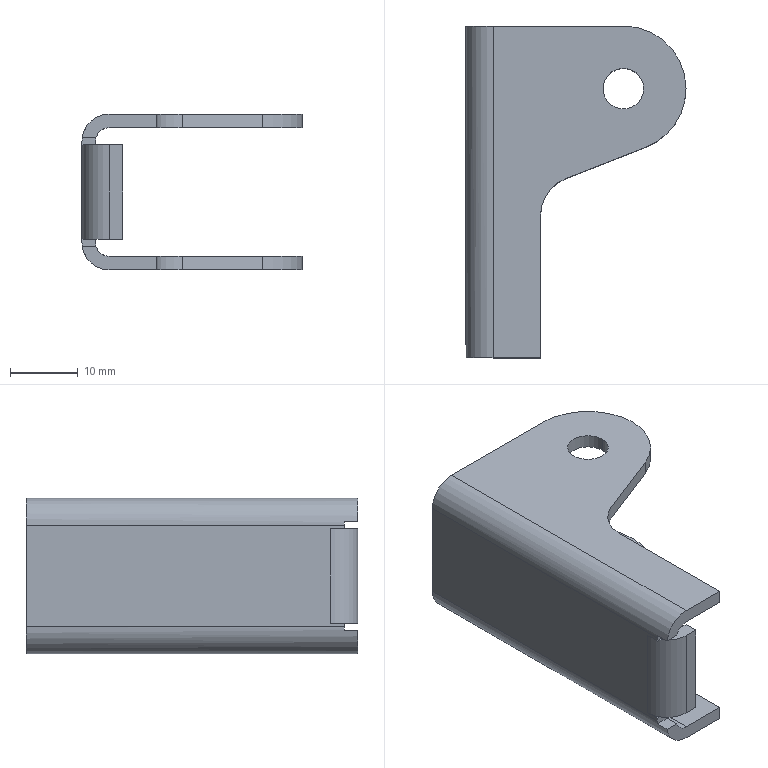Part | SolidWorks | features BaseBody 1 | 1 solid | 40 faces | box 32.5 x 49 x 23 mm | volume 5331 mm3 | plane 24 | cylinder 16 | commonest cylinder face diameters 6 x4 18.5 x4 4 x3 8 x3 12 x2
STEP:
#1=CARTESIAN_POINT('',(0.5359,2.,-7.));
#2=VERTEX_POINT('',#1);
#3=CARTESIAN_POINT('',(0.,4.,-7.));
#4=VERTEX_POINT('',#3);
#5=CARTESIAN_POINT('',(4.,4.,-7.));
#6=DIRECTION('',(0.,0.,-1.));
#7=DIRECTION('',(-0.866,-0.5,0.));
#8=AXIS2_PLACEMENT_3D('',#5,#6,#7);
#9=CIRCLE('',#8,4.);
#10=EDGE_CURVE('',#2,#4,#9,.T.);
#11=ORIENTED_EDGE('',*,*,#10,.T.);
#12=CARTESIAN_POINT('',(0.,2.,-7.));
#13=VERTEX_POINT('',#12);
#14=CARTESIAN_POINT('',(0.,4.,-7.));
#15=DIRECTION('',(0.,-1.,0.));
#16=VECTOR('',#15,1000.);
#17=LINE('',#14,#16);
#18=EDGE_CURVE('',#4,#13,#17,.T.);
#19=ORIENTED_EDGE('',*,*,#18,.T.);
#20=CARTESIAN_POINT('',(0.5359,2.,-7.));
#21=DIRECTION('',(-1.,0.,0.));
#22=VECTOR('',#21,1000.);
#23=LINE('',#20,#22);
#24=EDGE_CURVE('',#2,#13,#23,.T.);
#25=ORIENTED_EDGE('',*,*,#24,.F.);
#26=EDGE_LOOP('',(#11,#19,#25));
#27=FACE_OUTER_BOUND('',#26,.T.);
#28=CARTESIAN_POINT('',(0.,0.,-7.));
#29=DIRECTION('',(0.,0.,1.));
#30=DIRECTION('',(1.,0.,0.));
#31=AXIS2_PLACEMENT_3D('',#28,#29,#30);
#32=PLANE('',#31);
#33=ADVANCED_FACE('',(#27),#32,.T.);
#34=CARTESIAN_POINT('',(26.25,39.75,11.5));
#35=VERTEX_POINT('',#34);
#36=CARTESIAN_POINT('',(26.25,39.75,9.5));
#37=VERTEX_POINT('',#36);
#38=CARTESIAN_POINT('',(26.25,39.75,11.5));
#39=DIRECTION('',(0.,0.,-1.));
#40=VECTOR('',#39,1000.);
#41=LINE('',#38,#40);
#42=EDGE_CURVE('',#35,#37,#41,.T.);
#43=ORIENTED_EDGE('',*,*,#42,.T.);
#44=CARTESIAN_POINT('',(20.25,39.75,9.5));
#45=VERTEX_POINT('',#44);
#46=CARTESIAN_POINT('',(23.25,39.75,9.5));
#47=DIRECTION('',(0.,0.,1.));
#48=DIRECTION('',(-1.,0.,0.));
#49=AXIS2_PLACEMENT_3D('',#46,#47,#48);
#50=CIRCLE('',#49,3.);
#51=EDGE_CURVE('',#45,#37,#50,.T.);
#52=ORIENTED_EDGE('',*,*,#51,.F.);
#53=CARTESIAN_POINT('',(20.25,39.75,11.5));
#54=VERTEX_POINT('',#53);
#55=CARTESIAN_POINT('',(20.25,39.75,11.5));
#56=DIRECTION('',(0.,0.,-1.));
#57=VECTOR('',#56,1000.);
#58=LINE('',#55,#57);
#59=EDGE_CURVE('',#54,#45,#58,.T.);
#60=ORIENTED_EDGE('',*,*,#59,.F.);
#61=CARTESIAN_POINT('',(23.25,39.75,11.5));
#62=DIRECTION('',(0.,0.,1.));
#63=DIRECTION('',(-1.,0.,0.));
#64=AXIS2_PLACEMENT_3D('',#61,#62,#63);
#65=CIRCLE('',#64,3.);
#66=EDGE_CURVE('',#54,#35,#65,.T.);
#67=ORIENTED_EDGE('',*,*,#66,.T.);
#68=EDGE_LOOP('',(#43,#52,#60,#67));
#69=FACE_OUTER_BOUND('',#68,.T.);
#70=CARTESIAN_POINT('',(23.25,39.75,11.5));
#71=DIRECTION('',(0.,0.,1.));
#72=DIRECTION('',(1.,0.,0.));
#73=AXIS2_PLACEMENT_3D('',#70,#71,#72);
#74=CYLINDRICAL_SURFACE('',#73,3.);
#75=ADVANCED_FACE('',(#69),#74,.F.);
#76=CARTESIAN_POINT('',(20.25,39.75,-9.5));
#77=VERTEX_POINT('',#76);
#78=CARTESIAN_POINT('',(20.25,39.75,-11.5));
#79=VERTEX_POINT('',#78);
#80=CARTESIAN_POINT('',(20.25,39.75,-9.5));
#81=DIRECTION('',(0.,0.,-1.));
#82=VECTOR('',#81,1000.);
#83=LINE('',#80,#82);
#84=EDGE_CURVE('',#77,#79,#83,.T.);
#85=ORIENTED_EDGE('',*,*,#84,.F.);
#86=CARTESIAN_POINT('',(26.25,39.75,-9.5));
#87=VERTEX_POINT('',#86);
#88=CARTESIAN_POINT('',(23.25,39.75,-9.5));
#89=DIRECTION('',(0.,0.,1.));
#90=DIRECTION('',(-1.,0.,0.));
#91=AXIS2_PLACEMENT_3D('',#88,#89,#90);
#92=CIRCLE('',#91,3.);
#93=EDGE_CURVE('',#77,#87,#92,.T.);
#94=ORIENTED_EDGE('',*,*,#93,.T.);
#95=CARTESIAN_POINT('',(26.25,39.75,-11.5));
#96=VERTEX_POINT('',#95);
#97=CARTESIAN_POINT('',(26.25,39.75,-9.5));
#98=DIRECTION('',(0.,0.,-1.));
#99=VECTOR('',#98,1000.);
#100=LINE('',#97,#99);
#101=EDGE_CURVE('',#87,#96,#100,.T.);
#102=ORIENTED_EDGE('',*,*,#101,.T.);
#103=CARTESIAN_POINT('',(23.25,39.75,-11.5));
#104=DIRECTION('',(0.,0.,1.));
#105=DIRECTION('',(-1.,0.,0.));
#106=AXIS2_PLACEMENT_3D('',#103,#104,#105);
#107=CIRCLE('',#106,3.);
#108=EDGE_CURVE('',#79,#96,#107,.T.);
#109=ORIENTED_EDGE('',*,*,#108,.F.);
#110=EDGE_LOOP('',(#85,#94,#102,#109));
#111=FACE_OUTER_BOUND('',#110,.T.);
#112=CARTESIAN_POINT('',(23.25,39.75,11.5));
#113=DIRECTION('',(0.,0.,1.));
#114=DIRECTION('',(1.,0.,0.));
#115=AXIS2_PLACEMENT_3D('',#112,#113,#114);
#116=CYLINDRICAL_SURFACE('',#115,3.);
#117=ADVANCED_FACE('',(#111),#116,.F.);
#118=ORIENTED_EDGE('',*,*,#59,.T.);
#119=CARTESIAN_POINT('',(23.25,39.75,9.5));
#120=DIRECTION('',(0.,0.,1.));
#121=DIRECTION('',(1.,0.,0.));
#122=AXIS2_PLACEMENT_3D('',#119,#120,#121);
#123=CIRCLE('',#122,3.);
#124=EDGE_CURVE('',#37,#45,#123,.T.);
#125=ORIENTED_EDGE('',*,*,#124,.F.);
#126=ORIENTED_EDGE('',*,*,#42,.F.);
#127=CARTESIAN_POINT('',(23.25,39.75,11.5));
#128=DIRECTION('',(0.,0.,1.));
#129=DIRECTION('',(1.,0.,0.));
#130=AXIS2_PLACEMENT_3D('',#127,#128,#129);
#131=CIRCLE('',#130,3.);
#132=EDGE_CURVE('',#35,#54,#131,.T.);
#133=ORIENTED_EDGE('',*,*,#132,.T.);
#134=EDGE_LOOP('',(#118,#125,#126,#133));
#135=FACE_OUTER_BOUND('',#134,.T.);
#136=CARTESIAN_POINT('',(23.25,39.75,11.5));
#137=DIRECTION('',(0.,0.,1.));
#138=DIRECTION('',(1.,0.,0.));
#139=AXIS2_PLACEMENT_3D('',#136,#137,#138);
#140=CYLINDRICAL_SURFACE('',#139,3.);
#141=ADVANCED_FACE('',(#135),#140,.F.);
#142=ORIENTED_EDGE('',*,*,#101,.F.);
#143=CARTESIAN_POINT('',(23.25,39.75,-9.5));
#144=DIRECTION('',(0.,0.,1.));
#145=DIRECTION('',(1.,0.,0.));
#146=AXIS2_PLACEMENT_3D('',#143,#144,#145);
#147=CIRCLE('',#146,3.);
#148=EDGE_CURVE('',#87,#77,#147,.T.);
#149=ORIENTED_EDGE('',*,*,#148,.T.);
#150=ORIENTED_EDGE('',*,*,#84,.T.);
#151=CARTESIAN_POINT('',(23.25,39.75,-11.5));
#152=DIRECTION('',(0.,0.,1.));
#153=DIRECTION('',(1.,0.,0.));
#154=AXIS2_PLACEMENT_3D('',#151,#152,#153);
#155=CIRCLE('',#154,3.);
#156=EDGE_CURVE('',#96,#79,#155,.T.);
#157=ORIENTED_EDGE('',*,*,#156,.F.);
#158=EDGE_LOOP('',(#142,#149,#150,#157));
#159=FACE_OUTER_BOUND('',#158,.T.);
#160=CARTESIAN_POINT('',(23.25,39.75,11.5));
#161=DIRECTION('',(0.,0.,1.));
#162=DIRECTION('',(1.,0.,0.));
#163=AXIS2_PLACEMENT_3D('',#160,#161,#162);
#164=CYLINDRICAL_SURFACE('',#163,3.);
#165=ADVANCED_FACE('',(#159),#164,.F.);
#166=ORIENTED_EDGE('',*,*,#51,.T.);
#167=ORIENTED_EDGE('',*,*,#124,.T.);
#168=EDGE_LOOP('',(#166,#167));
#169=FACE_BOUND('',#168,.T.);
#170=CARTESIAN_POINT('',(11.,0.,9.5));
#171=VERTEX_POINT('',#170);
#172=CARTESIAN_POINT('',(4.,0.,9.5));
#173=VERTEX_POINT('',#172);
#174=CARTESIAN_POINT('',(11.,0.,9.5));
#175=DIRECTION('',(-1.,0.,0.));
#176=VECTOR('',#175,1000.);
#177=LINE('',#174,#176);
#178=EDGE_CURVE('',#171,#173,#177,.T.);
#179=ORIENTED_EDGE('',*,*,#178,.T.);
#180=CARTESIAN_POINT('',(4.,49.,9.5));
#181=VERTEX_POINT('',#180);
#182=CARTESIAN_POINT('',(4.,49.,9.5));
#183=DIRECTION('',(0.,-1.,0.));
#184=VECTOR('',#183,1000.);
#185=LINE('',#182,#184);
#186=EDGE_CURVE('',#181,#173,#185,.T.);
#187=ORIENTED_EDGE('',*,*,#186,.F.);
#188=CARTESIAN_POINT('',(23.25,49.,9.5));
#189=VERTEX_POINT('',#188);
#190=CARTESIAN_POINT('',(23.25,49.,9.5));
#191=DIRECTION('',(-1.,0.,0.));
#192=VECTOR('',#191,1000.);
#193=LINE('',#190,#192);
#194=EDGE_CURVE('',#189,#181,#193,.T.);
#195=ORIENTED_EDGE('',*,*,#194,.F.);
#196=CARTESIAN_POINT('',(32.5,39.75,9.5));
#197=VERTEX_POINT('',#196);
#198=CARTESIAN_POINT('',(23.25,39.75,9.5));
#199=DIRECTION('',(0.,0.,1.));
#200=DIRECTION('',(0.3656,-0.9308,0.));
#201=AXIS2_PLACEMENT_3D('',#198,#199,#200);
#202=CIRCLE('',#201,9.25);
#203=EDGE_CURVE('',#197,#189,#202,.T.);
#204=ORIENTED_EDGE('',*,*,#203,.F.);
#205=CARTESIAN_POINT('',(26.632,31.14,9.5));
#206=VERTEX_POINT('',#205);
#207=CARTESIAN_POINT('',(23.25,39.75,9.5));
#208=DIRECTION('',(0.,0.,1.));
#209=DIRECTION('',(0.3656,-0.9308,0.));
#210=AXIS2_PLACEMENT_3D('',#207,#208,#209);
#211=CIRCLE('',#210,9.25);
#212=EDGE_CURVE('',#206,#197,#211,.T.);
#213=ORIENTED_EDGE('',*,*,#212,.F.);
#214=CARTESIAN_POINT('',(14.806,26.495,9.5));
#215=VERTEX_POINT('',#214);
#216=CARTESIAN_POINT('',(14.806,26.495,9.5));
#217=DIRECTION('',(0.9308,0.3656,0.));
#218=VECTOR('',#217,1000.);
#219=LINE('',#216,#218);
#220=EDGE_CURVE('',#215,#206,#219,.T.);
#221=ORIENTED_EDGE('',*,*,#220,.F.);
#222=CARTESIAN_POINT('',(11.,20.911,9.5));
#223=VERTEX_POINT('',#222);
#224=CARTESIAN_POINT('',(17.,20.911,9.5));
#225=DIRECTION('',(0.,0.,1.));
#226=DIRECTION('',(-0.3656,0.9308,0.));
#227=AXIS2_PLACEMENT_3D('',#224,#225,#226);
#228=CIRCLE('',#227,6.);
#229=EDGE_CURVE('',#215,#223,#228,.T.);
#230=ORIENTED_EDGE('',*,*,#229,.T.);
#231=CARTESIAN_POINT('',(11.,0.,9.5));
#232=DIRECTION('',(0.,1.,0.));
#233=VECTOR('',#232,1000.);
#234=LINE('',#231,#233);
#235=EDGE_CURVE('',#171,#223,#234,.T.);
#236=ORIENTED_EDGE('',*,*,#235,.F.);
#237=EDGE_LOOP('',(#179,#187,#195,#204,#213,#221,#230,#236));
#238=FACE_OUTER_BOUND('',#237,.T.);
#239=CARTESIAN_POINT('',(0.,0.,9.5));
#240=DIRECTION('',(0.,0.,1.));
#241=DIRECTION('',(1.,0.,0.));
#242=AXIS2_PLACEMENT_3D('',#239,#240,#241);
#243=PLANE('',#242);
#244=ADVANCED_FACE('',(#169,#238),#243,.F.);
#245=CARTESIAN_POINT('',(32.5,39.75,11.5));
#246=VERTEX_POINT('',#245);
#247=CARTESIAN_POINT('',(32.5,39.75,-11.5));
#248=DIRECTION('',(0.,0.,1.));
#249=VECTOR('',#248,1000.);
#250=LINE('',#247,#249);
#251=EDGE_CURVE('',#197,#246,#250,.T.);
#252=ORIENTED_EDGE('',*,*,#251,.F.);
#253=ORIENTED_EDGE('',*,*,#203,.T.);
#254=CARTESIAN_POINT('',(23.25,49.,11.5));
#255=VERTEX_POINT('',#254);
#256=CARTESIAN_POINT('',(23.25,49.,9.5));
#257=DIRECTION('',(0.,0.,1.));
#258=VECTOR('',#257,1000.);
#259=LINE('',#256,#258);
#260=EDGE_CURVE('',#189,#255,#259,.T.);
#261=ORIENTED_EDGE('',*,*,#260,.T.);
#262=CARTESIAN_POINT('',(23.25,39.75,11.5));
#263=DIRECTION('',(0.,0.,1.));
#264=DIRECTION('',(0.3656,-0.9308,0.));
#265=AXIS2_PLACEMENT_3D('',#262,#263,#264);
#266=CIRCLE('',#265,9.25);
#267=EDGE_CURVE('',#246,#255,#266,.T.);
#268=ORIENTED_EDGE('',*,*,#267,.F.);
#269=EDGE_LOOP('',(#252,#253,#261,#268));
#270=FACE_OUTER_BOUND('',#269,.T.);
#271=CARTESIAN_POINT('',(23.25,39.75,-11.5));
#272=DIRECTION('',(0.,0.,1.));
#273=DIRECTION('',(1.,0.,0.));
#274=AXIS2_PLACEMENT_3D('',#271,#272,#273);
#275=CYLINDRICAL_SURFACE('',#274,9.25);
#276=ADVANCED_FACE('',(#270),#275,.T.);
#277=CARTESIAN_POINT('',(32.5,39.75,-11.5));
#278=VERTEX_POINT('',#277);
#279=CARTESIAN_POINT('',(32.5,39.75,-9.5));
#280=VERTEX_POINT('',#279);
#281=CARTESIAN_POINT('',(32.5,39.75,-11.5));
#282=DIRECTION('',(0.,0.,1.));
#283=VECTOR('',#282,1000.);
#284=LINE('',#281,#283);
#285=EDGE_CURVE('',#278,#280,#284,.T.);
#286=ORIENTED_EDGE('',*,*,#285,.F.);
#287=CARTESIAN_POINT('',(23.25,49.,-11.5));
#288=VERTEX_POINT('',#287);
#289=CARTESIAN_POINT('',(23.25,39.75,-11.5));
#290=DIRECTION('',(0.,0.,1.));
#291=DIRECTION('',(0.3656,-0.9308,0.));
#292=AXIS2_PLACEMENT_3D('',#289,#290,#291);
#293=CIRCLE('',#292,9.25);
#294=EDGE_CURVE('',#278,#288,#293,.T.);
#295=ORIENTED_EDGE('',*,*,#294,.T.);
#296=CARTESIAN_POINT('',(23.25,49.,-9.5));
#297=VERTEX_POINT('',#296);
#298=CARTESIAN_POINT('',(23.25,49.,-11.5));
#299=DIRECTION('',(0.,0.,1.));
#300=VECTOR('',#299,1000.);
#301=LINE('',#298,#300);
#302=EDGE_CURVE('',#288,#297,#301,.T.);
#303=ORIENTED_EDGE('',*,*,#302,.T.);
#304=CARTESIAN_POINT('',(23.25,39.75,-9.5));
#305=DIRECTION('',(0.,0.,1.));
#306=DIRECTION('',(0.3656,-0.9308,0.));
#307=AXIS2_PLACEMENT_3D('',#304,#305,#306);
#308=CIRCLE('',#307,9.25);
#309=EDGE_CURVE('',#280,#297,#308,.T.);
#310=ORIENTED_EDGE('',*,*,#309,.F.);
#311=EDGE_LOOP('',(#286,#295,#303,#310));
#312=FACE_OUTER_BOUND('',#311,.T.);
#313=CARTESIAN_POINT('',(23.25,39.75,-11.5));
#314=DIRECTION('',(0.,0.,1.));
#315=DIRECTION('',(1.,0.,0.));
#316=AXIS2_PLACEMENT_3D('',#313,#314,#315);
#317=CYLINDRICAL_SURFACE('',#316,9.25);
#318=ADVANCED_FACE('',(#312),#317,.T.);
#319=CARTESIAN_POINT('',(11.,20.911,-9.5));
#320=VERTEX_POINT('',#319);
#321=CARTESIAN_POINT('',(14.806,26.495,-9.5));
#322=VERTEX_POINT('',#321);
#323=CARTESIAN_POINT('',(17.,20.911,-9.5));
#324=DIRECTION('',(0.,0.,-1.));
#325=DIRECTION('',(-1.,0.,0.));
#326=AXIS2_PLACEMENT_3D('',#323,#324,#325);
#327=CIRCLE('',#326,6.);
#328=EDGE_CURVE('',#320,#322,#327,.T.);
#329=ORIENTED_EDGE('',*,*,#328,.F.);
#330=CARTESIAN_POINT('',(11.,20.911,-11.5));
#331=VERTEX_POINT('',#330);
#332=CARTESIAN_POINT('',(11.,20.911,-11.5));
#333=DIRECTION('',(0.,0.,1.));
#334=VECTOR('',#333,1000.);
#335=LINE('',#332,#334);
#336=EDGE_CURVE('',#331,#320,#335,.T.);
#337=ORIENTED_EDGE('',*,*,#336,.F.);
#338=CARTESIAN_POINT('',(14.806,26.495,-11.5));
#339=VERTEX_POINT('',#338);
#340=CARTESIAN_POINT('',(17.,20.911,-11.5));
#341=DIRECTION('',(0.,0.,1.));
#342=DIRECTION('',(-0.3656,0.9308,0.));
#343=AXIS2_PLACEMENT_3D('',#340,#341,#342);
#344=CIRCLE('',#343,6.);
#345=EDGE_CURVE('',#339,#331,#344,.T.);
#346=ORIENTED_EDGE('',*,*,#345,.F.);
#347=CARTESIAN_POINT('',(14.806,26.495,-11.5));
#348=DIRECTION('',(0.,0.,1.));
#349=VECTOR('',#348,1000.);
#350=LINE('',#347,#349);
#351=EDGE_CURVE('',#339,#322,#350,.T.);
#352=ORIENTED_EDGE('',*,*,#351,.T.);
#353=EDGE_LOOP('',(#329,#337,#346,#352));
#354=FACE_OUTER_BOUND('',#353,.T.);
#355=CARTESIAN_POINT('',(17.,20.911,-41.483));
#356=DIRECTION('',(0.,0.,1.));
#357=DIRECTION('',(-0.3656,0.9308,0.));
#358=AXIS2_PLACEMENT_3D('',#355,#356,#357);
#359=CYLINDRICAL_SURFACE('',#358,6.);
#360=ADVANCED_FACE('',(#354),#359,.F.);
#361=ORIENTED_EDGE('',*,*,#93,.F.);
#362=ORIENTED_EDGE('',*,*,#148,.F.);
#363=EDGE_LOOP('',(#361,#362));
#364=FACE_BOUND('',#363,.T.);
#365=CARTESIAN_POINT('',(26.632,31.14,-9.5));
#366=VERTEX_POINT('',#365);
#367=CARTESIAN_POINT('',(23.25,39.75,-9.5));
#368=DIRECTION('',(0.,0.,1.));
#369=DIRECTION('',(0.3656,-0.9308,0.));
#370=AXIS2_PLACEMENT_3D('',#367,#368,#369);
#371=CIRCLE('',#370,9.25);
#372=EDGE_CURVE('',#366,#280,#371,.T.);
#373=ORIENTED_EDGE('',*,*,#372,.T.);
#374=ORIENTED_EDGE('',*,*,#309,.T.);
#375=CARTESIAN_POINT('',(4.,49.,-9.5));
#376=VERTEX_POINT('',#375);
#377=CARTESIAN_POINT('',(23.25,49.,-9.5));
#378=DIRECTION('',(-1.,0.,0.));
#379=VECTOR('',#378,1000.);
#380=LINE('',#377,#379);
#381=EDGE_CURVE('',#297,#376,#380,.T.);
#382=ORIENTED_EDGE('',*,*,#381,.T.);
#383=CARTESIAN_POINT('',(4.,0.,-9.5));
#384=VERTEX_POINT('',#383);
#385=CARTESIAN_POINT('',(4.,0.,-9.5));
#386=DIRECTION('',(0.,1.,0.));
#387=VECTOR('',#386,1000.);
#388=LINE('',#385,#387);
#389=EDGE_CURVE('',#384,#376,#388,.T.);
#390=ORIENTED_EDGE('',*,*,#389,.F.);
#391=CARTESIAN_POINT('',(11.,0.,-9.5));
#392=VERTEX_POINT('',#391);
#393=CARTESIAN_POINT('',(11.,0.,-9.5));
#394=DIRECTION('',(-1.,0.,0.));
#395=VECTOR('',#394,1000.);
#396=LINE('',#393,#395);
#397=EDGE_CURVE('',#392,#384,#396,.T.);
#398=ORIENTED_EDGE('',*,*,#397,.F.);
#399=CARTESIAN_POINT('',(11.,0.,-9.5));
#400=DIRECTION('',(0.,1.,0.));
#401=VECTOR('',#400,1000.);
#402=LINE('',#399,#401);
#403=EDGE_CURVE('',#392,#320,#402,.T.);
#404=ORIENTED_EDGE('',*,*,#403,.T.);
#405=ORIENTED_EDGE('',*,*,#328,.T.);
#406=CARTESIAN_POINT('',(14.806,26.495,-9.5));
#407=DIRECTION('',(0.9308,0.3656,0.));
#408=VECTOR('',#407,1000.);
#409=LINE('',#406,#408);
#410=EDGE_CURVE('',#322,#366,#409,.T.);
#411=ORIENTED_EDGE('',*,*,#410,.T.);
#412=EDGE_LOOP('',(#373,#374,#382,#390,#398,#404,#405,#411));
#413=FACE_OUTER_BOUND('',#412,.T.);
#414=CARTESIAN_POINT('',(0.,0.,-9.5));
#415=DIRECTION('',(0.,0.,1.));
#416=DIRECTION('',(1.,0.,0.));
#417=AXIS2_PLACEMENT_3D('',#414,#415,#416);
#418=PLANE('',#417);
#419=ADVANCED_FACE('',(#364,#413),#418,.T.);
#420=CARTESIAN_POINT('',(2.064,0.,-8.));
#421=VERTEX_POINT('',#420);
#422=CARTESIAN_POINT('',(2.064,2.,-8.));
#423=VERTEX_POINT('',#422);
#424=CARTESIAN_POINT('',(2.064,0.,-8.));
#425=DIRECTION('',(0.,1.,0.));
#426=VECTOR('',#425,1000.);
#427=LINE('',#424,#426);
#428=EDGE_CURVE('',#421,#423,#427,.T.);
#429=ORIENTED_EDGE('',*,*,#428,.F.);
#430=CARTESIAN_POINT('',(4.,0.,-7.5));
#431=DIRECTION('',(0.,1.,0.));
#432=DIRECTION('',(0.,0.,-1.));
#433=AXIS2_PLACEMENT_3D('',#430,#431,#432);
#434=CIRCLE('',#433,2.);
#435=EDGE_CURVE('',#384,#421,#434,.T.);
#436=ORIENTED_EDGE('',*,*,#435,.F.);
#437=ORIENTED_EDGE('',*,*,#389,.T.);
#438=CARTESIAN_POINT('',(2.,49.,-7.5));
#439=VERTEX_POINT('',#438);
#440=CARTESIAN_POINT('',(4.,49.,-7.5));
#441=DIRECTION('',(0.,-1.,0.));
#442=DIRECTION('',(-1.,0.,0.));
#443=AXIS2_PLACEMENT_3D('',#440,#441,#442);
#444=CIRCLE('',#443,2.);
#445=EDGE_CURVE('',#439,#376,#444,.T.);
#446=ORIENTED_EDGE('',*,*,#445,.F.);
#447=CARTESIAN_POINT('',(2.,2.,-7.5));
#448=VERTEX_POINT('',#447);
#449=CARTESIAN_POINT('',(2.,2.,-7.5));
#450=DIRECTION('',(0.,1.,0.));
#451=VECTOR('',#450,1000.);
#452=LINE('',#449,#451);
#453=EDGE_CURVE('',#448,#439,#452,.T.);
#454=ORIENTED_EDGE('',*,*,#453,.F.);
#455=CARTESIAN_POINT('',(4.,2.,-7.5));
#456=DIRECTION('',(0.,1.,0.));
#457=DIRECTION('',(-0.9682,0.,-0.25));
#458=AXIS2_PLACEMENT_3D('',#455,#456,#457);
#459=CIRCLE('',#458,2.);
#460=EDGE_CURVE('',#423,#448,#459,.T.);
#461=ORIENTED_EDGE('',*,*,#460,.F.);
#462=EDGE_LOOP('',(#429,#436,#437,#446,#454,#461));
#463=FACE_OUTER_BOUND('',#462,.T.);
#464=CARTESIAN_POINT('',(4.,-63.876,-7.5));
#465=DIRECTION('',(0.,1.,0.));
#466=DIRECTION('',(0.,0.,-1.));
#467=AXIS2_PLACEMENT_3D('',#464,#465,#466);
#468=CYLINDRICAL_SURFACE('',#467,2.);
#469=ADVANCED_FACE('',(#463),#468,.F.);
#470=ORIENTED_EDGE('',*,*,#428,.T.);
#471=CARTESIAN_POINT('',(0.03137,2.,-8.));
#472=VERTEX_POINT('',#471);
#473=CARTESIAN_POINT('',(0.03137,2.,-8.));
#474=DIRECTION('',(1.,0.,0.));
#475=VECTOR('',#474,1000.);
#476=LINE('',#473,#475);
#477=EDGE_CURVE('',#472,#423,#476,.T.);
#478=ORIENTED_EDGE('',*,*,#477,.F.);
#479=CARTESIAN_POINT('',(0.03137,0.,-8.));
#480=VERTEX_POINT('',#479);
#481=CARTESIAN_POINT('',(0.03137,0.,-8.));
#482=DIRECTION('',(0.,1.,0.));
#483=VECTOR('',#482,1000.);
#484=LINE('',#481,#483);
#485=EDGE_CURVE('',#480,#472,#484,.T.);
#486=ORIENTED_EDGE('',*,*,#485,.F.);
#487=CARTESIAN_POINT('',(0.03137,0.,-8.));
#488=DIRECTION('',(1.,0.,0.));
#489=VECTOR('',#488,1000.);
#490=LINE('',#487,#489);
#491=EDGE_CURVE('',#480,#421,#490,.T.);
#492=ORIENTED_EDGE('',*,*,#491,.T.);
#493=EDGE_LOOP('',(#470,#478,#486,#492));
#494=FACE_OUTER_BOUND('',#493,.T.);
#495=CARTESIAN_POINT('',(0.,0.,-8.));
#496=DIRECTION('',(0.,0.,-1.));
#497=DIRECTION('',(0.,-1.,0.));
#498=AXIS2_PLACEMENT_3D('',#495,#496,#497);
#499=PLANE('',#498);
#500=ADVANCED_FACE('',(#494),#499,.F.);
#501=CARTESIAN_POINT('',(0.,2.,-7.5));
#502=VERTEX_POINT('',#501);
#503=CARTESIAN_POINT('',(0.,49.,-7.5));
#504=VERTEX_POINT('',#503);
#505=CARTESIAN_POINT('',(0.,2.,-7.5));
#506=DIRECTION('',(0.,1.,0.));
#507=VECTOR('',#506,1000.);
#508=LINE('',#505,#507);
#509=EDGE_CURVE('',#502,#504,#508,.T.);
#510=ORIENTED_EDGE('',*,*,#509,.T.);
#511=CARTESIAN_POINT('',(4.,49.,-11.5));
#512=VERTEX_POINT('',#511);
#513=CARTESIAN_POINT('',(4.,49.,-7.5));
#514=DIRECTION('',(0.,1.,0.));
#515=DIRECTION('',(0.,0.,-1.));
#516=AXIS2_PLACEMENT_3D('',#513,#514,#515);
#517=CIRCLE('',#516,4.);
#518=EDGE_CURVE('',#512,#504,#517,.T.);
#519=ORIENTED_EDGE('',*,*,#518,.F.);
#520=CARTESIAN_POINT('',(4.,0.,-11.5));
#521=VERTEX_POINT('',#520);
#522=CARTESIAN_POINT('',(4.,0.,-11.5));
#523=DIRECTION('',(0.,1.,0.));
#524=VECTOR('',#523,1000.);
#525=LINE('',#522,#524);
#526=EDGE_CURVE('',#521,#512,#525,.T.);
#527=ORIENTED_EDGE('',*,*,#526,.F.);
#528=CARTESIAN_POINT('',(4.,0.,-7.5));
#529=DIRECTION('',(0.,-1.,0.));
#530=DIRECTION('',(-0.9922,0.,-0.125));
#531=AXIS2_PLACEMENT_3D('',#528,#529,#530);
#532=CIRCLE('',#531,4.);
#533=EDGE_CURVE('',#480,#521,#532,.T.);
#534=ORIENTED_EDGE('',*,*,#533,.F.);
#535=ORIENTED_EDGE('',*,*,#485,.T.);
#536=CARTESIAN_POINT('',(4.,2.,-7.5));
#537=DIRECTION('',(0.,1.,0.));
#538=DIRECTION('',(-0.9922,0.,-0.125));
#539=AXIS2_PLACEMENT_3D('',#536,#537,#538);
#540=CIRCLE('',#539,4.);
#541=EDGE_CURVE('',#472,#502,#540,.T.);
#542=ORIENTED_EDGE('',*,*,#541,.T.);
#543=EDGE_LOOP('',(#510,#519,#527,#534,#535,#542));
#544=FACE_OUTER_BOUND('',#543,.T.);
#545=CARTESIAN_POINT('',(4.,-63.876,-7.5));
#546=DIRECTION('',(0.,1.,0.));
#547=DIRECTION('',(0.,0.,-1.));
#548=AXIS2_PLACEMENT_3D('',#545,#546,#547);
#549=CYLINDRICAL_SURFACE('',#548,4.);
#550=ADVANCED_FACE('',(#544),#549,.T.);
#551=CARTESIAN_POINT('',(0.03137,2.,8.));
#552=VERTEX_POINT('',#551);
#553=CARTESIAN_POINT('',(0.03137,0.,8.));
#554=VERTEX_POINT('',#553);
#555=CARTESIAN_POINT('',(0.03137,2.,8.));
#556=DIRECTION('',(0.,-1.,0.));
#557=VECTOR('',#556,1000.);
#558=LINE('',#555,#557);
#559=EDGE_CURVE('',#552,#554,#558,.T.);
#560=ORIENTED_EDGE('',*,*,#559,.T.);
#561=CARTESIAN_POINT('',(4.,0.,11.5));
#562=VERTEX_POINT('',#561);
#563=CARTESIAN_POINT('',(4.,0.,7.5));
#564=DIRECTION('',(0.,-1.,0.));
#565=DIRECTION('',(0.,0.,1.));
#566=AXIS2_PLACEMENT_3D('',#563,#564,#565);
#567=CIRCLE('',#566,4.);
#568=EDGE_CURVE('',#562,#554,#567,.T.);
#569=ORIENTED_EDGE('',*,*,#568,.F.);
#570=CARTESIAN_POINT('',(4.,49.,11.5));
#571=VERTEX_POINT('',#570);
#572=CARTESIAN_POINT('',(4.,49.,11.5));
#573=DIRECTION('',(0.,-1.,0.));
#574=VECTOR('',#573,1000.);
#575=LINE('',#572,#574);
#576=EDGE_CURVE('',#571,#562,#575,.T.);
#577=ORIENTED_EDGE('',*,*,#576,.F.);
#578=CARTESIAN_POINT('',(0.,49.,7.5));
#579=VERTEX_POINT('',#578);
#580=CARTESIAN_POINT('',(4.,49.,7.5));
#581=DIRECTION('',(0.,1.,0.));
#582=DIRECTION('',(-1.,0.,0.));
#583=AXIS2_PLACEMENT_3D('',#580,#581,#582);
#584=CIRCLE('',#583,4.);
#585=EDGE_CURVE('',#579,#571,#584,.T.);
#586=ORIENTED_EDGE('',*,*,#585,.F.);
#587=CARTESIAN_POINT('',(0.,2.,7.5));
#588=VERTEX_POINT('',#587);
#589=CARTESIAN_POINT('',(0.,49.,7.5));
#590=DIRECTION('',(0.,-1.,0.));
#591=VECTOR('',#590,1000.);
#592=LINE('',#589,#591);
#593=EDGE_CURVE('',#579,#588,#592,.T.);
#594=ORIENTED_EDGE('',*,*,#593,.T.);
#595=CARTESIAN_POINT('',(4.,2.,7.5));
#596=DIRECTION('',(0.,-1.,0.));
#597=DIRECTION('',(-0.9922,0.,0.125));
#598=AXIS2_PLACEMENT_3D('',#595,#596,#597);
#599=CIRCLE('',#598,4.);
#600=EDGE_CURVE('',#552,#588,#599,.T.);
#601=ORIENTED_EDGE('',*,*,#600,.F.);
#602=EDGE_LOOP('',(#560,#569,#577,#586,#594,#601));
#603=FACE_OUTER_BOUND('',#602,.T.);
#604=CARTESIAN_POINT('',(4.,112.876,7.5));
#605=DIRECTION('',(0.,-1.,0.));
#606=DIRECTION('',(0.,0.,1.));
#607=AXIS2_PLACEMENT_3D('',#604,#605,#606);
#608=CYLINDRICAL_SURFACE('',#607,4.);
#609=ADVANCED_FACE('',(#603),#608,.T.);
#610=CARTESIAN_POINT('',(23.25,49.,11.5));
#611=DIRECTION('',(-1.,0.,0.));
#612=VECTOR('',#611,1000.);
#613=LINE('',#610,#612);
#614=EDGE_CURVE('',#255,#571,#613,.T.);
#615=ORIENTED_EDGE('',*,*,#614,.F.);
#616=ORIENTED_EDGE('',*,*,#260,.F.);
#617=ORIENTED_EDGE('',*,*,#194,.T.);
#618=CARTESIAN_POINT('',(2.,49.,7.5));
#619=VERTEX_POINT('',#618);
#620=CARTESIAN_POINT('',(4.,49.,7.5));
#621=DIRECTION('',(0.,-1.,0.));
#622=DIRECTION('',(0.,0.,1.));
#623=AXIS2_PLACEMENT_3D('',#620,#621,#622);
#624=CIRCLE('',#623,2.);
#625=EDGE_CURVE('',#181,#619,#624,.T.);
#626=ORIENTED_EDGE('',*,*,#625,.T.);
#627=CARTESIAN_POINT('',(2.,49.,-7.5));
#628=DIRECTION('',(0.,0.,1.));
#629=VECTOR('',#628,1000.);
#630=LINE('',#627,#629);
#631=EDGE_CURVE('',#439,#619,#630,.T.);
#632=ORIENTED_EDGE('',*,*,#631,.F.);
#633=ORIENTED_EDGE('',*,*,#445,.T.);
#634=ORIENTED_EDGE('',*,*,#381,.F.);
#635=ORIENTED_EDGE('',*,*,#302,.F.);
#636=CARTESIAN_POINT('',(23.25,49.,-11.5));
#637=DIRECTION('',(-1.,0.,0.));
#638=VECTOR('',#637,1000.);
#639=LINE('',#636,#638);
#640=EDGE_CURVE('',#288,#512,#639,.T.);
#641=ORIENTED_EDGE('',*,*,#640,.T.);
#642=ORIENTED_EDGE('',*,*,#518,.T.);
#643=CARTESIAN_POINT('',(0.,49.,-7.5));
#644=DIRECTION('',(0.,0.,1.));
#645=VECTOR('',#644,1000.);
#646=LINE('',#643,#645);
#647=EDGE_CURVE('',#504,#579,#646,.T.);
#648=ORIENTED_EDGE('',*,*,#647,.T.);
#649=ORIENTED_EDGE('',*,*,#585,.T.);
#650=EDGE_LOOP('',(#615,#616,#617,#626,#632,#633,#634,#635,#641,#642,#648,#649));
#651=FACE_OUTER_BOUND('',#650,.T.);
#652=CARTESIAN_POINT('',(23.25,49.,-11.5));
#653=DIRECTION('',(0.,1.,0.));
#654=DIRECTION('',(1.,0.,0.));
#655=AXIS2_PLACEMENT_3D('',#652,#653,#654);
#656=PLANE('',#655);
#657=ADVANCED_FACE('',(#651),#656,.T.);
#658=CARTESIAN_POINT('',(6.,2.,7.));
#659=VERTEX_POINT('',#658);
#660=CARTESIAN_POINT('',(4.,2.,7.));
#661=VERTEX_POINT('',#660);
#662=CARTESIAN_POINT('',(6.,2.,7.));
#663=DIRECTION('',(-1.,0.,0.));
#664=VECTOR('',#663,1000.);
#665=LINE('',#662,#664);
#666=EDGE_CURVE('',#659,#661,#665,.T.);
#667=ORIENTED_EDGE('',*,*,#666,.F.);
#668=CARTESIAN_POINT('',(6.,2.,-7.));
#669=VERTEX_POINT('',#668);
#670=CARTESIAN_POINT('',(6.,2.,-7.));
#671=DIRECTION('',(0.,0.,1.));
#672=VECTOR('',#671,1000.);
#673=LINE('',#670,#672);
#674=EDGE_CURVE('',#669,#659,#673,.T.);
#675=ORIENTED_EDGE('',*,*,#674,.F.);
#676=CARTESIAN_POINT('',(4.,2.,-7.));
#677=VERTEX_POINT('',#676);
#678=CARTESIAN_POINT('',(6.,2.,-7.));
#679=DIRECTION('',(-1.,0.,0.));
#680=VECTOR('',#679,1000.);
#681=LINE('',#678,#680);
#682=EDGE_CURVE('',#669,#677,#681,.T.);
#683=ORIENTED_EDGE('',*,*,#682,.T.);
#684=CARTESIAN_POINT('',(4.,2.,-7.));
#685=DIRECTION('',(0.,0.,1.));
#686=VECTOR('',#685,1000.);
#687=LINE('',#684,#686);
#688=EDGE_CURVE('',#677,#661,#687,.T.);
#689=ORIENTED_EDGE('',*,*,#688,.T.);
#690=EDGE_LOOP('',(#667,#675,#683,#689));
#691=FACE_OUTER_BOUND('',#690,.T.);
#692=CARTESIAN_POINT('',(6.,2.,-7.));
#693=DIRECTION('',(0.,1.,0.));
#694=DIRECTION('',(1.,0.,0.));
#695=AXIS2_PLACEMENT_3D('',#692,#693,#694);
#696=PLANE('',#695);
#697=ADVANCED_FACE('',(#691),#696,.T.);
#698=CARTESIAN_POINT('',(2.,4.,7.));
#699=VERTEX_POINT('',#698);
#700=CARTESIAN_POINT('',(4.,4.,7.));
#701=DIRECTION('',(0.,0.,-1.));
#702=DIRECTION('',(0.,-1.,0.));
#703=AXIS2_PLACEMENT_3D('',#700,#701,#702);
#704=CIRCLE('',#703,2.);
#705=EDGE_CURVE('',#661,#699,#704,.T.);
#706=ORIENTED_EDGE('',*,*,#705,.F.);
#707=ORIENTED_EDGE('',*,*,#688,.F.);
#708=CARTESIAN_POINT('',(2.,4.,-7.));
#709=VERTEX_POINT('',#708);
#710=CARTESIAN_POINT('',(4.,4.,-7.));
#711=DIRECTION('',(0.,0.,1.));
#712=DIRECTION('',(-1.,0.,0.));
#713=AXIS2_PLACEMENT_3D('',#710,#711,#712);
#714=CIRCLE('',#713,2.);
#715=EDGE_CURVE('',#709,#677,#714,.T.);
#716=ORIENTED_EDGE('',*,*,#715,.F.);
#717=CARTESIAN_POINT('',(2.,4.,-7.));
#718=DIRECTION('',(0.,0.,1.));
#719=VECTOR('',#718,1000.);
#720=LINE('',#717,#719);
#721=EDGE_CURVE('',#709,#699,#720,.T.);
#722=ORIENTED_EDGE('',*,*,#721,.T.);
#723=EDGE_LOOP('',(#706,#707,#716,#722));
#724=FACE_OUTER_BOUND('',#723,.T.);
#725=CARTESIAN_POINT('',(4.,4.,-41.483));
#726=DIRECTION('',(0.,0.,1.));
#727=DIRECTION('',(-1.,0.,0.));
#728=AXIS2_PLACEMENT_3D('',#725,#726,#727);
#729=CYLINDRICAL_SURFACE('',#728,2.);
#730=ADVANCED_FACE('',(#724),#729,.F.);
#731=ORIENTED_EDGE('',*,*,#453,.T.);
#732=ORIENTED_EDGE('',*,*,#631,.T.);
#733=CARTESIAN_POINT('',(2.,2.,7.5));
#734=VERTEX_POINT('',#733);
#735=CARTESIAN_POINT('',(2.,49.,7.5));
#736=DIRECTION('',(0.,-1.,0.));
#737=VECTOR('',#736,1000.);
#738=LINE('',#735,#737);
#739=EDGE_CURVE('',#619,#734,#738,.T.);
#740=ORIENTED_EDGE('',*,*,#739,.T.);
#741=CARTESIAN_POINT('',(2.,2.,7.));
#742=VERTEX_POINT('',#741);
#743=CARTESIAN_POINT('',(2.,2.,7.));
#744=DIRECTION('',(0.,0.,1.));
#745=VECTOR('',#744,1000.);
#746=LINE('',#743,#745);
#747=EDGE_CURVE('',#742,#734,#746,.T.);
#748=ORIENTED_EDGE('',*,*,#747,.F.);
#749=CARTESIAN_POINT('',(2.,2.,7.));
#750=DIRECTION('',(0.,1.,0.));
#751=VECTOR('',#750,1000.);
#752=LINE('',#749,#751);
#753=EDGE_CURVE('',#742,#699,#752,.T.);
#754=ORIENTED_EDGE('',*,*,#753,.T.);
#755=ORIENTED_EDGE('',*,*,#721,.F.);
#756=CARTESIAN_POINT('',(2.,2.,-7.));
#757=VERTEX_POINT('',#756);
#758=CARTESIAN_POINT('',(2.,4.,-7.));
#759=DIRECTION('',(0.,-1.,0.));
#760=VECTOR('',#759,1000.);
#761=LINE('',#758,#760);
#762=EDGE_CURVE('',#709,#757,#761,.T.);
#763=ORIENTED_EDGE('',*,*,#762,.T.);
#764=CARTESIAN_POINT('',(2.,2.,-7.5));
#765=DIRECTION('',(0.,0.,1.));
#766=VECTOR('',#765,1000.);
#767=LINE('',#764,#766);
#768=EDGE_CURVE('',#448,#757,#767,.T.);
#769=ORIENTED_EDGE('',*,*,#768,.F.);
#770=EDGE_LOOP('',(#731,#732,#740,#748,#754,#755,#763,#769));
#771=FACE_OUTER_BOUND('',#770,.T.);
#772=CARTESIAN_POINT('',(2.,49.,-11.5));
#773=DIRECTION('',(-1.,0.,0.));
#774=DIRECTION('',(0.,0.,1.));
#775=AXIS2_PLACEMENT_3D('',#772,#773,#774);
#776=PLANE('',#775);
#777=ADVANCED_FACE('',(#771),#776,.F.);
#778=CARTESIAN_POINT('',(6.,0.,7.));
#779=VERTEX_POINT('',#778);
#780=CARTESIAN_POINT('',(4.,0.,7.));
#781=VERTEX_POINT('',#780);
#782=CARTESIAN_POINT('',(6.,0.,7.));
#783=DIRECTION('',(-1.,0.,0.));
#784=VECTOR('',#783,1000.);
#785=LINE('',#782,#784);
#786=EDGE_CURVE('',#779,#781,#785,.T.);
#787=ORIENTED_EDGE('',*,*,#786,.F.);
#788=CARTESIAN_POINT('',(6.,0.,7.));
#789=DIRECTION('',(0.,1.,0.));
#790=VECTOR('',#789,1000.);
#791=LINE('',#788,#790);
#792=EDGE_CURVE('',#779,#659,#791,.T.);
#793=ORIENTED_EDGE('',*,*,#792,.T.);
#794=ORIENTED_EDGE('',*,*,#666,.T.);
#795=ORIENTED_EDGE('',*,*,#705,.T.);
#796=ORIENTED_EDGE('',*,*,#753,.F.);
#797=CARTESIAN_POINT('',(0.5359,2.,7.));
#798=VERTEX_POINT('',#797);
#799=CARTESIAN_POINT('',(0.5359,2.,7.));
#800=DIRECTION('',(1.,0.,0.));
#801=VECTOR('',#800,1000.);
#802=LINE('',#799,#801);
#803=EDGE_CURVE('',#798,#742,#802,.T.);
#804=ORIENTED_EDGE('',*,*,#803,.F.);
#805=CARTESIAN_POINT('',(4.,4.,7.));
#806=DIRECTION('',(0.,0.,1.));
#807=DIRECTION('',(-0.866,-0.5,0.));
#808=AXIS2_PLACEMENT_3D('',#805,#806,#807);
#809=CIRCLE('',#808,4.);
#810=EDGE_CURVE('',#798,#781,#809,.T.);
#811=ORIENTED_EDGE('',*,*,#810,.T.);
#812=EDGE_LOOP('',(#787,#793,#794,#795,#796,#804,#811));
#813=FACE_OUTER_BOUND('',#812,.T.);
#814=CARTESIAN_POINT('',(0.,0.,7.));
#815=DIRECTION('',(0.,0.,1.));
#816=DIRECTION('',(1.,0.,0.));
#817=AXIS2_PLACEMENT_3D('',#814,#815,#816);
#818=PLANE('',#817);
#819=ADVANCED_FACE('',(#813),#818,.T.);
#820=ORIENTED_EDGE('',*,*,#674,.T.);
#821=ORIENTED_EDGE('',*,*,#792,.F.);
#822=CARTESIAN_POINT('',(6.,0.,-7.));
#823=VERTEX_POINT('',#822);
#824=CARTESIAN_POINT('',(6.,0.,-7.));
#825=DIRECTION('',(0.,0.,1.));
#826=VECTOR('',#825,1000.);
#827=LINE('',#824,#826);
#828=EDGE_CURVE('',#823,#779,#827,.T.);
#829=ORIENTED_EDGE('',*,*,#828,.F.);
#830=CARTESIAN_POINT('',(6.,0.,-7.));
#831=DIRECTION('',(0.,1.,0.));
#832=VECTOR('',#831,1000.);
#833=LINE('',#830,#832);
#834=EDGE_CURVE('',#823,#669,#833,.T.);
#835=ORIENTED_EDGE('',*,*,#834,.T.);
#836=EDGE_LOOP('',(#820,#821,#829,#835));
#837=FACE_OUTER_BOUND('',#836,.T.);
#838=CARTESIAN_POINT('',(6.,0.,-7.));
#839=DIRECTION('',(1.,0.,0.));
#840=DIRECTION('',(0.,1.,0.));
#841=AXIS2_PLACEMENT_3D('',#838,#839,#840);
#842=PLANE('',#841);
#843=ADVANCED_FACE('',(#837),#842,.T.);
#844=CARTESIAN_POINT('',(2.,2.,-7.));
#845=DIRECTION('',(-1.,0.,0.));
#846=VECTOR('',#845,1000.);
#847=LINE('',#844,#846);
#848=EDGE_CURVE('',#757,#2,#847,.T.);
#849=ORIENTED_EDGE('',*,*,#848,.F.);
#850=ORIENTED_EDGE('',*,*,#762,.F.);
#851=ORIENTED_EDGE('',*,*,#715,.T.);
#852=ORIENTED_EDGE('',*,*,#682,.F.);
#853=ORIENTED_EDGE('',*,*,#834,.F.);
#854=CARTESIAN_POINT('',(4.,0.,-7.));
#855=VERTEX_POINT('',#854);
#856=CARTESIAN_POINT('',(4.,0.,-7.));
#857=DIRECTION('',(1.,0.,0.));
#858=VECTOR('',#857,1000.);
#859=LINE('',#856,#858);
#860=EDGE_CURVE('',#855,#823,#859,.T.);
#861=ORIENTED_EDGE('',*,*,#860,.F.);
#862=CARTESIAN_POINT('',(4.,4.,-7.));
#863=DIRECTION('',(0.,0.,-1.));
#864=DIRECTION('',(0.,-1.,0.));
#865=AXIS2_PLACEMENT_3D('',#862,#863,#864);
#866=CIRCLE('',#865,4.);
#867=EDGE_CURVE('',#855,#2,#866,.T.);
#868=ORIENTED_EDGE('',*,*,#867,.T.);
#869=EDGE_LOOP('',(#849,#850,#851,#852,#853,#861,#868));
#870=FACE_OUTER_BOUND('',#869,.T.);
#871=CARTESIAN_POINT('',(0.,0.,-7.));
#872=DIRECTION('',(0.,0.,1.));
#873=DIRECTION('',(1.,0.,0.));
#874=AXIS2_PLACEMENT_3D('',#871,#872,#873);
#875=PLANE('',#874);
#876=ADVANCED_FACE('',(#870),#875,.F.);
#877=CARTESIAN_POINT('',(4.,0.,7.));
#878=DIRECTION('',(0.,0.,-1.));
#879=VECTOR('',#878,1000.);
#880=LINE('',#877,#879);
#881=EDGE_CURVE('',#781,#855,#880,.T.);
#882=ORIENTED_EDGE('',*,*,#881,.F.);
#883=ORIENTED_EDGE('',*,*,#810,.F.);
#884=CARTESIAN_POINT('',(0.,4.,7.));
#885=VERTEX_POINT('',#884);
#886=CARTESIAN_POINT('',(4.,4.,7.));
#887=DIRECTION('',(0.,0.,1.));
#888=DIRECTION('',(-1.,0.,0.));
#889=AXIS2_PLACEMENT_3D('',#886,#887,#888);
#890=CIRCLE('',#889,4.);
#891=EDGE_CURVE('',#885,#798,#890,.T.);
#892=ORIENTED_EDGE('',*,*,#891,.F.);
#893=CARTESIAN_POINT('',(0.,4.,7.));
#894=DIRECTION('',(0.,0.,-1.));
#895=VECTOR('',#894,1000.);
#896=LINE('',#893,#895);
#897=EDGE_CURVE('',#885,#4,#896,.T.);
#898=ORIENTED_EDGE('',*,*,#897,.T.);
#899=ORIENTED_EDGE('',*,*,#10,.F.);
#900=ORIENTED_EDGE('',*,*,#867,.F.);
#901=EDGE_LOOP('',(#882,#883,#892,#898,#899,#900));
#902=FACE_OUTER_BOUND('',#901,.T.);
#903=CARTESIAN_POINT('',(4.,4.,41.483));
#904=DIRECTION('',(0.,0.,-1.));
#905=DIRECTION('',(0.,-1.,0.));
#906=AXIS2_PLACEMENT_3D('',#903,#904,#905);
#907=CYLINDRICAL_SURFACE('',#906,4.);
#908=ADVANCED_FACE('',(#902),#907,.T.);
#909=CARTESIAN_POINT('',(0.,2.,7.));
#910=VERTEX_POINT('',#909);
#911=CARTESIAN_POINT('',(0.,4.,7.));
#912=DIRECTION('',(0.,-1.,0.));
#913=VECTOR('',#912,1000.);
#914=LINE('',#911,#913);
#915=EDGE_CURVE('',#885,#910,#914,.T.);
#916=ORIENTED_EDGE('',*,*,#915,.T.);
#917=CARTESIAN_POINT('',(0.,2.,7.));
#918=DIRECTION('',(0.,0.,1.));
#919=VECTOR('',#918,1000.);
#920=LINE('',#917,#919);
#921=EDGE_CURVE('',#910,#588,#920,.T.);
#922=ORIENTED_EDGE('',*,*,#921,.T.);
#923=ORIENTED_EDGE('',*,*,#593,.F.);
#924=ORIENTED_EDGE('',*,*,#647,.F.);
#925=ORIENTED_EDGE('',*,*,#509,.F.);
#926=CARTESIAN_POINT('',(0.,2.,-7.5));
#927=DIRECTION('',(0.,0.,1.));
#928=VECTOR('',#927,1000.);
#929=LINE('',#926,#928);
#930=EDGE_CURVE('',#502,#13,#929,.T.);
#931=ORIENTED_EDGE('',*,*,#930,.T.);
#932=ORIENTED_EDGE('',*,*,#18,.F.);
#933=ORIENTED_EDGE('',*,*,#897,.F.);
#934=EDGE_LOOP('',(#916,#922,#923,#924,#925,#931,#932,#933));
#935=FACE_OUTER_BOUND('',#934,.T.);
#936=CARTESIAN_POINT('',(0.,49.,-11.5));
#937=DIRECTION('',(-1.,0.,0.));
#938=DIRECTION('',(0.,0.,1.));
#939=AXIS2_PLACEMENT_3D('',#936,#937,#938);
#940=PLANE('',#939);
#941=ADVANCED_FACE('',(#935),#940,.T.);
#942=ORIENTED_EDGE('',*,*,#891,.T.);
#943=CARTESIAN_POINT('',(0.,2.,7.));
#944=DIRECTION('',(1.,0.,0.));
#945=VECTOR('',#944,1000.);
#946=LINE('',#943,#945);
#947=EDGE_CURVE('',#910,#798,#946,.T.);
#948=ORIENTED_EDGE('',*,*,#947,.F.);
#949=ORIENTED_EDGE('',*,*,#915,.F.);
#950=EDGE_LOOP('',(#942,#948,#949));
#951=FACE_OUTER_BOUND('',#950,.T.);
#952=CARTESIAN_POINT('',(0.,0.,7.));
#953=DIRECTION('',(0.,0.,1.));
#954=DIRECTION('',(1.,0.,0.));
#955=AXIS2_PLACEMENT_3D('',#952,#953,#954);
#956=PLANE('',#955);
#957=ADVANCED_FACE('',(#951),#956,.F.);
#958=ORIENTED_EDGE('',*,*,#930,.F.);
#959=ORIENTED_EDGE('',*,*,#541,.F.);
#960=ORIENTED_EDGE('',*,*,#477,.T.);
#961=ORIENTED_EDGE('',*,*,#460,.T.);
#962=ORIENTED_EDGE('',*,*,#768,.T.);
#963=ORIENTED_EDGE('',*,*,#848,.T.);
#964=ORIENTED_EDGE('',*,*,#24,.T.);
#965=EDGE_LOOP('',(#958,#959,#960,#961,#962,#963,#964));
#966=FACE_OUTER_BOUND('',#965,.T.);
#967=CARTESIAN_POINT('',(0.,2.,-11.5));
#968=DIRECTION('',(0.,-1.,0.));
#969=DIRECTION('',(0.,0.,-1.));
#970=AXIS2_PLACEMENT_3D('',#967,#968,#969);
#971=PLANE('',#970);
#972=ADVANCED_FACE('',(#966),#971,.T.);
#973=ORIENTED_EDGE('',*,*,#803,.T.);
#974=ORIENTED_EDGE('',*,*,#747,.T.);
#975=CARTESIAN_POINT('',(2.064,2.,8.));
#976=VERTEX_POINT('',#975);
#977=CARTESIAN_POINT('',(4.,2.,7.5));
#978=DIRECTION('',(0.,-1.,0.));
#979=DIRECTION('',(-0.9682,0.,0.25));
#980=AXIS2_PLACEMENT_3D('',#977,#978,#979);
#981=CIRCLE('',#980,2.);
#982=EDGE_CURVE('',#976,#734,#981,.T.);
#983=ORIENTED_EDGE('',*,*,#982,.F.);
#984=CARTESIAN_POINT('',(2.064,2.,8.));
#985=DIRECTION('',(-1.,0.,0.));
#986=VECTOR('',#985,1000.);
#987=LINE('',#984,#986);
#988=EDGE_CURVE('',#976,#552,#987,.T.);
#989=ORIENTED_EDGE('',*,*,#988,.T.);
#990=ORIENTED_EDGE('',*,*,#600,.T.);
#991=ORIENTED_EDGE('',*,*,#921,.F.);
#992=ORIENTED_EDGE('',*,*,#947,.T.);
#993=EDGE_LOOP('',(#973,#974,#983,#989,#990,#991,#992));
#994=FACE_OUTER_BOUND('',#993,.T.);
#995=CARTESIAN_POINT('',(0.,2.,-11.5));
#996=DIRECTION('',(0.,-1.,0.));
#997=DIRECTION('',(0.,0.,-1.));
#998=AXIS2_PLACEMENT_3D('',#995,#996,#997);
#999=PLANE('',#998);
#1000=ADVANCED_FACE('',(#994),#999,.T.);
#1001=ORIENTED_EDGE('',*,*,#739,.F.);
#1002=ORIENTED_EDGE('',*,*,#625,.F.);
#1003=ORIENTED_EDGE('',*,*,#186,.T.);
#1004=CARTESIAN_POINT('',(2.064,0.,8.));
#1005=VERTEX_POINT('',#1004);
#1006=CARTESIAN_POINT('',(4.,0.,7.5));
#1007=DIRECTION('',(0.,1.,0.));
#1008=DIRECTION('',(-0.9682,0.,0.25));
#1009=AXIS2_PLACEMENT_3D('',#1006,#1007,#1008);
#1010=CIRCLE('',#1009,2.);
#1011=EDGE_CURVE('',#1005,#173,#1010,.T.);
#1012=ORIENTED_EDGE('',*,*,#1011,.F.);
#1013=CARTESIAN_POINT('',(2.064,2.,8.));
#1014=DIRECTION('',(0.,-1.,0.));
#1015=VECTOR('',#1014,1000.);
#1016=LINE('',#1013,#1015);
#1017=EDGE_CURVE('',#976,#1005,#1016,.T.);
#1018=ORIENTED_EDGE('',*,*,#1017,.F.);
#1019=ORIENTED_EDGE('',*,*,#982,.T.);
#1020=EDGE_LOOP('',(#1001,#1002,#1003,#1012,#1018,#1019));
#1021=FACE_OUTER_BOUND('',#1020,.T.);
#1022=CARTESIAN_POINT('',(4.,112.876,7.5));
#1023=DIRECTION('',(0.,-1.,0.));
#1024=DIRECTION('',(0.,0.,1.));
#1025=AXIS2_PLACEMENT_3D('',#1022,#1023,#1024);
#1026=CYLINDRICAL_SURFACE('',#1025,2.);
#1027=ADVANCED_FACE('',(#1021),#1026,.F.);
#1028=ORIENTED_EDGE('',*,*,#559,.F.);
#1029=ORIENTED_EDGE('',*,*,#988,.F.);
#1030=ORIENTED_EDGE('',*,*,#1017,.T.);
#1031=CARTESIAN_POINT('',(0.03137,0.,8.));
#1032=DIRECTION('',(1.,0.,0.));
#1033=VECTOR('',#1032,1000.);
#1034=LINE('',#1031,#1033);
#1035=EDGE_CURVE('',#554,#1005,#1034,.T.);
#1036=ORIENTED_EDGE('',*,*,#1035,.F.);
#1037=EDGE_LOOP('',(#1028,#1029,#1030,#1036));
#1038=FACE_OUTER_BOUND('',#1037,.T.);
#1039=CARTESIAN_POINT('',(2.5,0.,8.));
#1040=DIRECTION('',(0.,0.,1.));
#1041=DIRECTION('',(1.,0.,0.));
#1042=AXIS2_PLACEMENT_3D('',#1039,#1040,#1041);
#1043=PLANE('',#1042);
#1044=ADVANCED_FACE('',(#1038),#1043,.F.);
#1045=ORIENTED_EDGE('',*,*,#860,.T.);
#1046=ORIENTED_EDGE('',*,*,#828,.T.);
#1047=ORIENTED_EDGE('',*,*,#786,.T.);
#1048=ORIENTED_EDGE('',*,*,#881,.T.);
#1049=EDGE_LOOP('',(#1045,#1046,#1047,#1048));
#1050=FACE_OUTER_BOUND('',#1049,.T.);
#1051=CARTESIAN_POINT('',(0.,0.,-11.5));
#1052=DIRECTION('',(0.,-1.,0.));
#1053=DIRECTION('',(0.,0.,-1.));
#1054=AXIS2_PLACEMENT_3D('',#1051,#1052,#1053);
#1055=PLANE('',#1054);
#1056=ADVANCED_FACE('',(#1050),#1055,.T.);
#1057=ORIENTED_EDGE('',*,*,#533,.T.);
#1058=CARTESIAN_POINT('',(11.,0.,-11.5));
#1059=VERTEX_POINT('',#1058);
#1060=CARTESIAN_POINT('',(4.,0.,-11.5));
#1061=DIRECTION('',(1.,0.,0.));
#1062=VECTOR('',#1061,1000.);
#1063=LINE('',#1060,#1062);
#1064=EDGE_CURVE('',#521,#1059,#1063,.T.);
#1065=ORIENTED_EDGE('',*,*,#1064,.T.);
#1066=CARTESIAN_POINT('',(11.,0.,-11.5));
#1067=DIRECTION('',(0.,0.,1.));
#1068=VECTOR('',#1067,1000.);
#1069=LINE('',#1066,#1068);
#1070=EDGE_CURVE('',#1059,#392,#1069,.T.);
#1071=ORIENTED_EDGE('',*,*,#1070,.T.);
#1072=ORIENTED_EDGE('',*,*,#397,.T.);
#1073=ORIENTED_EDGE('',*,*,#435,.T.);
#1074=ORIENTED_EDGE('',*,*,#491,.F.);
#1075=EDGE_LOOP('',(#1057,#1065,#1071,#1072,#1073,#1074));
#1076=FACE_OUTER_BOUND('',#1075,.T.);
#1077=CARTESIAN_POINT('',(0.,0.,-11.5));
#1078=DIRECTION('',(0.,-1.,0.));
#1079=DIRECTION('',(0.,0.,-1.));
#1080=AXIS2_PLACEMENT_3D('',#1077,#1078,#1079);
#1081=PLANE('',#1080);
#1082=ADVANCED_FACE('',(#1076),#1081,.T.);
#1083=ORIENTED_EDGE('',*,*,#1011,.T.);
#1084=ORIENTED_EDGE('',*,*,#178,.F.);
#1085=CARTESIAN_POINT('',(11.,0.,11.5));
#1086=VERTEX_POINT('',#1085);
#1087=CARTESIAN_POINT('',(11.,0.,9.5));
#1088=DIRECTION('',(0.,0.,1.));
#1089=VECTOR('',#1088,1000.);
#1090=LINE('',#1087,#1089);
#1091=EDGE_CURVE('',#171,#1086,#1090,.T.);
#1092=ORIENTED_EDGE('',*,*,#1091,.T.);
#1093=CARTESIAN_POINT('',(4.,0.,11.5));
#1094=DIRECTION('',(1.,0.,0.));
#1095=VECTOR('',#1094,1000.);
#1096=LINE('',#1093,#1095);
#1097=EDGE_CURVE('',#562,#1086,#1096,.T.);
#1098=ORIENTED_EDGE('',*,*,#1097,.F.);
#1099=ORIENTED_EDGE('',*,*,#568,.T.);
#1100=ORIENTED_EDGE('',*,*,#1035,.T.);
#1101=EDGE_LOOP('',(#1083,#1084,#1092,#1098,#1099,#1100));
#1102=FACE_OUTER_BOUND('',#1101,.T.);
#1103=CARTESIAN_POINT('',(0.,0.,-11.5));
#1104=DIRECTION('',(0.,-1.,0.));
#1105=DIRECTION('',(0.,0.,-1.));
#1106=AXIS2_PLACEMENT_3D('',#1103,#1104,#1105);
#1107=PLANE('',#1106);
#1108=ADVANCED_FACE('',(#1102),#1107,.T.);
#1109=ORIENTED_EDGE('',*,*,#66,.F.);
#1110=ORIENTED_EDGE('',*,*,#132,.F.);
#1111=EDGE_LOOP('',(#1109,#1110));
#1112=FACE_BOUND('',#1111,.T.);
#1113=CARTESIAN_POINT('',(26.632,31.14,11.5));
#1114=VERTEX_POINT('',#1113);
#1115=CARTESIAN_POINT('',(23.25,39.75,11.5));
#1116=DIRECTION('',(0.,0.,1.));
#1117=DIRECTION('',(0.3656,-0.9308,0.));
#1118=AXIS2_PLACEMENT_3D('',#1115,#1116,#1117);
#1119=CIRCLE('',#1118,9.25);
#1120=EDGE_CURVE('',#1114,#246,#1119,.T.);
#1121=ORIENTED_EDGE('',*,*,#1120,.T.);
#1122=ORIENTED_EDGE('',*,*,#267,.T.);
#1123=ORIENTED_EDGE('',*,*,#614,.T.);
#1124=ORIENTED_EDGE('',*,*,#576,.T.);
#1125=ORIENTED_EDGE('',*,*,#1097,.T.);
#1126=CARTESIAN_POINT('',(11.,20.911,11.5));
#1127=VERTEX_POINT('',#1126);
#1128=CARTESIAN_POINT('',(11.,0.,11.5));
#1129=DIRECTION('',(0.,1.,0.));
#1130=VECTOR('',#1129,1000.);
#1131=LINE('',#1128,#1130);
#1132=EDGE_CURVE('',#1086,#1127,#1131,.T.);
#1133=ORIENTED_EDGE('',*,*,#1132,.T.);
#1134=CARTESIAN_POINT('',(14.806,26.495,11.5));
#1135=VERTEX_POINT('',#1134);
#1136=CARTESIAN_POINT('',(17.,20.911,11.5));
#1137=DIRECTION('',(0.,0.,-1.));
#1138=DIRECTION('',(-1.,0.,0.));
#1139=AXIS2_PLACEMENT_3D('',#1136,#1137,#1138);
#1140=CIRCLE('',#1139,6.);
#1141=EDGE_CURVE('',#1127,#1135,#1140,.T.);
#1142=ORIENTED_EDGE('',*,*,#1141,.T.);
#1143=CARTESIAN_POINT('',(14.806,26.495,11.5));
#1144=DIRECTION('',(0.9308,0.3656,0.));
#1145=VECTOR('',#1144,1000.);
#1146=LINE('',#1143,#1145);
#1147=EDGE_CURVE('',#1135,#1114,#1146,.T.);
#1148=ORIENTED_EDGE('',*,*,#1147,.T.);
#1149=EDGE_LOOP('',(#1121,#1122,#1123,#1124,#1125,#1133,#1142,#1148));
#1150=FACE_OUTER_BOUND('',#1149,.T.);
#1151=CARTESIAN_POINT('',(0.,0.,11.5));
#1152=DIRECTION('',(0.,0.,1.));
#1153=DIRECTION('',(1.,0.,0.));
#1154=AXIS2_PLACEMENT_3D('',#1151,#1152,#1153);
#1155=PLANE('',#1154);
#1156=ADVANCED_FACE('',(#1112,#1150),#1155,.T.);
#1157=CARTESIAN_POINT('',(26.632,31.14,-11.5));
#1158=VERTEX_POINT('',#1157);
#1159=CARTESIAN_POINT('',(14.806,26.495,-11.5));
#1160=DIRECTION('',(0.9308,0.3656,0.));
#1161=VECTOR('',#1160,1000.);
#1162=LINE('',#1159,#1161);
#1163=EDGE_CURVE('',#339,#1158,#1162,.T.);
#1164=ORIENTED_EDGE('',*,*,#1163,.T.);
#1165=CARTESIAN_POINT('',(26.632,31.14,-11.5));
#1166=DIRECTION('',(0.,0.,1.));
#1167=VECTOR('',#1166,1000.);
#1168=LINE('',#1165,#1167);
#1169=EDGE_CURVE('',#1158,#366,#1168,.T.);
#1170=ORIENTED_EDGE('',*,*,#1169,.T.);
#1171=ORIENTED_EDGE('',*,*,#410,.F.);
#1172=ORIENTED_EDGE('',*,*,#351,.F.);
#1173=EDGE_LOOP('',(#1164,#1170,#1171,#1172));
#1174=FACE_OUTER_BOUND('',#1173,.T.);
#1175=CARTESIAN_POINT('',(11.,25.,-11.5));
#1176=DIRECTION('',(0.3656,-0.9308,0.));
#1177=DIRECTION('',(0.,0.,-1.));
#1178=AXIS2_PLACEMENT_3D('',#1175,#1176,#1177);
#1179=PLANE('',#1178);
#1180=ADVANCED_FACE('',(#1174),#1179,.T.);
#1181=ORIENTED_EDGE('',*,*,#220,.T.);
#1182=CARTESIAN_POINT('',(26.632,31.14,9.5));
#1183=DIRECTION('',(0.,0.,1.));
#1184=VECTOR('',#1183,1000.);
#1185=LINE('',#1182,#1184);
#1186=EDGE_CURVE('',#206,#1114,#1185,.T.);
#1187=ORIENTED_EDGE('',*,*,#1186,.T.);
#1188=ORIENTED_EDGE('',*,*,#1147,.F.);
#1189=CARTESIAN_POINT('',(14.806,26.495,9.5));
#1190=DIRECTION('',(0.,0.,1.));
#1191=VECTOR('',#1190,1000.);
#1192=LINE('',#1189,#1191);
#1193=EDGE_CURVE('',#215,#1135,#1192,.T.);
#1194=ORIENTED_EDGE('',*,*,#1193,.F.);
#1195=EDGE_LOOP('',(#1181,#1187,#1188,#1194));
#1196=FACE_OUTER_BOUND('',#1195,.T.);
#1197=CARTESIAN_POINT('',(11.,25.,-11.5));
#1198=DIRECTION('',(0.3656,-0.9308,0.));
#1199=DIRECTION('',(0.,0.,-1.));
#1200=AXIS2_PLACEMENT_3D('',#1197,#1198,#1199);
#1201=PLANE('',#1200);
#1202=ADVANCED_FACE('',(#1196),#1201,.T.);
#1203=ORIENTED_EDGE('',*,*,#1141,.F.);
#1204=CARTESIAN_POINT('',(11.,20.911,9.5));
#1205=DIRECTION('',(0.,0.,1.));
#1206=VECTOR('',#1205,1000.);
#1207=LINE('',#1204,#1206);
#1208=EDGE_CURVE('',#223,#1127,#1207,.T.);
#1209=ORIENTED_EDGE('',*,*,#1208,.F.);
#1210=ORIENTED_EDGE('',*,*,#229,.F.);
#1211=ORIENTED_EDGE('',*,*,#1193,.T.);
#1212=EDGE_LOOP('',(#1203,#1209,#1210,#1211));
#1213=FACE_OUTER_BOUND('',#1212,.T.);
#1214=CARTESIAN_POINT('',(17.,20.911,-41.483));
#1215=DIRECTION('',(0.,0.,1.));
#1216=DIRECTION('',(-0.3656,0.9308,0.));
#1217=AXIS2_PLACEMENT_3D('',#1214,#1215,#1216);
#1218=CYLINDRICAL_SURFACE('',#1217,6.);
#1219=ADVANCED_FACE('',(#1213),#1218,.F.);
#1220=ORIENTED_EDGE('',*,*,#403,.F.);
#1221=ORIENTED_EDGE('',*,*,#1070,.F.);
#1222=CARTESIAN_POINT('',(11.,0.,-11.5));
#1223=DIRECTION('',(0.,1.,0.));
#1224=VECTOR('',#1223,1000.);
#1225=LINE('',#1222,#1224);
#1226=EDGE_CURVE('',#1059,#331,#1225,.T.);
#1227=ORIENTED_EDGE('',*,*,#1226,.T.);
#1228=ORIENTED_EDGE('',*,*,#336,.T.);
#1229=EDGE_LOOP('',(#1220,#1221,#1227,#1228));
#1230=FACE_OUTER_BOUND('',#1229,.T.);
#1231=CARTESIAN_POINT('',(11.,0.,-11.5));
#1232=DIRECTION('',(1.,0.,0.));
#1233=DIRECTION('',(0.,1.,0.));
#1234=AXIS2_PLACEMENT_3D('',#1231,#1232,#1233);
#1235=PLANE('',#1234);
#1236=ADVANCED_FACE('',(#1230),#1235,.T.);
#1237=ORIENTED_EDGE('',*,*,#1132,.F.);
#1238=ORIENTED_EDGE('',*,*,#1091,.F.);
#1239=ORIENTED_EDGE('',*,*,#235,.T.);
#1240=ORIENTED_EDGE('',*,*,#1208,.T.);
#1241=EDGE_LOOP('',(#1237,#1238,#1239,#1240));
#1242=FACE_OUTER_BOUND('',#1241,.T.);
#1243=CARTESIAN_POINT('',(11.,0.,-11.5));
#1244=DIRECTION('',(1.,0.,0.));
#1245=DIRECTION('',(0.,1.,0.));
#1246=AXIS2_PLACEMENT_3D('',#1243,#1244,#1245);
#1247=PLANE('',#1246);
#1248=ADVANCED_FACE('',(#1242),#1247,.T.);
#1249=ORIENTED_EDGE('',*,*,#108,.T.);
#1250=ORIENTED_EDGE('',*,*,#156,.T.);
#1251=EDGE_LOOP('',(#1249,#1250));
#1252=FACE_BOUND('',#1251,.T.);
#1253=ORIENTED_EDGE('',*,*,#1064,.F.);
#1254=ORIENTED_EDGE('',*,*,#526,.T.);
#1255=ORIENTED_EDGE('',*,*,#640,.F.);
#1256=ORIENTED_EDGE('',*,*,#294,.F.);
#1257=CARTESIAN_POINT('',(23.25,39.75,-11.5));
#1258=DIRECTION('',(0.,0.,1.));
#1259=DIRECTION('',(0.3656,-0.9308,0.));
#1260=AXIS2_PLACEMENT_3D('',#1257,#1258,#1259);
#1261=CIRCLE('',#1260,9.25);
#1262=EDGE_CURVE('',#1158,#278,#1261,.T.);
#1263=ORIENTED_EDGE('',*,*,#1262,.F.);
#1264=ORIENTED_EDGE('',*,*,#1163,.F.);
#1265=ORIENTED_EDGE('',*,*,#345,.T.);
#1266=ORIENTED_EDGE('',*,*,#1226,.F.);
#1267=EDGE_LOOP('',(#1253,#1254,#1255,#1256,#1263,#1264,#1265,#1266));
#1268=FACE_OUTER_BOUND('',#1267,.T.);
#1269=CARTESIAN_POINT('',(0.,0.,-11.5));
#1270=DIRECTION('',(0.,0.,1.));
#1271=DIRECTION('',(1.,0.,0.));
#1272=AXIS2_PLACEMENT_3D('',#1269,#1270,#1271);
#1273=PLANE('',#1272);
#1274=ADVANCED_FACE('',(#1252,#1268),#1273,.F.);
#1275=ORIENTED_EDGE('',*,*,#1262,.T.);
#1276=ORIENTED_EDGE('',*,*,#285,.T.);
#1277=ORIENTED_EDGE('',*,*,#372,.F.);
#1278=ORIENTED_EDGE('',*,*,#1169,.F.);
#1279=EDGE_LOOP('',(#1275,#1276,#1277,#1278));
#1280=FACE_OUTER_BOUND('',#1279,.T.);
#1281=CARTESIAN_POINT('',(23.25,39.75,-11.5));
#1282=DIRECTION('',(0.,0.,1.));
#1283=DIRECTION('',(1.,0.,0.));
#1284=AXIS2_PLACEMENT_3D('',#1281,#1282,#1283);
#1285=CYLINDRICAL_SURFACE('',#1284,9.25);
#1286=ADVANCED_FACE('',(#1280),#1285,.T.);
#1287=ORIENTED_EDGE('',*,*,#212,.T.);
#1288=ORIENTED_EDGE('',*,*,#251,.T.);
#1289=ORIENTED_EDGE('',*,*,#1120,.F.);
#1290=ORIENTED_EDGE('',*,*,#1186,.F.);
#1291=EDGE_LOOP('',(#1287,#1288,#1289,#1290));
#1292=FACE_OUTER_BOUND('',#1291,.T.);
#1293=CARTESIAN_POINT('',(23.25,39.75,-11.5));
#1294=DIRECTION('',(0.,0.,1.));
#1295=DIRECTION('',(1.,0.,0.));
#1296=AXIS2_PLACEMENT_3D('',#1293,#1294,#1295);
#1297=CYLINDRICAL_SURFACE('',#1296,9.25);
#1298=ADVANCED_FACE('',(#1292),#1297,.T.);
#1299=CLOSED_SHELL('',(#33,#75,#117,#141,#165,#244,#276,#318,#360,#419,#469,#500,#550,#609,#657,#697,#730,#777,#819,#843,#876,#908,#941,#957,#972,#1000,#1027,#1044,#1056,#1082,#1108,#1156,#1180,#1202,#1219,#1236,#1248,#1274,#1286,#1298));
#1300=MANIFOLD_SOLID_BREP('',#1299);
#1301=CARTESIAN_POINT('',(0.,0.,0.));
#1302=DIRECTION('',(0.,0.,1.));
#1303=DIRECTION('',(1.,0.,0.));
#1304=AXIS2_PLACEMENT_3D('',#1301,#1302,#1303);
#1305=(LENGTH_UNIT()NAMED_UNIT(*)SI_UNIT(.MILLI.,.METRE.));
#1306=UNCERTAINTY_MEASURE_WITH_UNIT(LENGTH_MEASURE(0.00001),#1305,'','');
#1307=(NAMED_UNIT(*)PLANE_ANGLE_UNIT()SI_UNIT($,.RADIAN.));
#1308=(NAMED_UNIT(*)SI_UNIT($,.STERADIAN.)SOLID_ANGLE_UNIT());
#1309=(GEOMETRIC_REPRESENTATION_CONTEXT(3)GLOBAL_UNCERTAINTY_ASSIGNED_CONTEXT((#1306))GLOBAL_UNIT_ASSIGNED_CONTEXT((#1305,#1307,#1308))REPRESENTATION_CONTEXT('',''));
#1310=ADVANCED_BREP_SHAPE_REPRESENTATION('',(#1300,#1304),#1309);